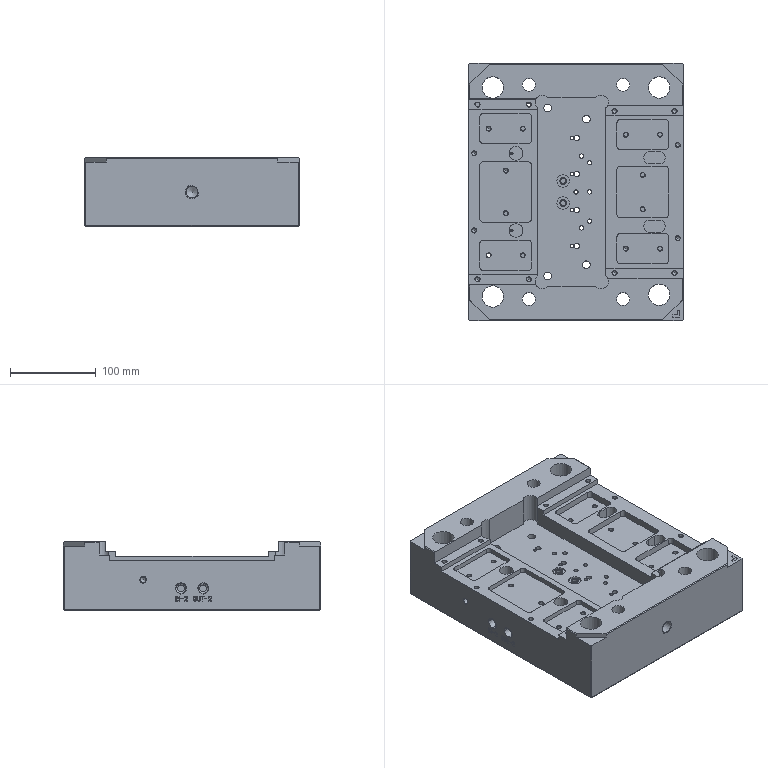NC program | PowerMill | posted with a generic post | part box 250 x 300 x 80 mm
Whole program:
%
O0001
N104 ( POWERMILL CB  : 2026004.0)
N105 ( POST VER      : 2026.0.0.5161)
N106 ( OPTION FILE   : FANUC)
N107 ( OUTPUT WORKPLANE : 1)
N108 (  )
N109 ( TOOL LIST )
N110 (-----------------------------------)
N111 ( NO. | ID    | DIA.| TIP RAD|LENGTH)
N112 (-----------------------------------)
N113 (    1|￠6_1_1| 6.0 |  0.0   |139.96)
N114 (-----------------------------------)
N115 (  )
N116 ( NUMBER OF TOOLPATHS: 1.0 )
N117 ( ESTIMATED PROGRAM DURATION: 0 HOURS 3 MIN 57 SEC)
N118 (  )
N119 G00 G21 G80 G40 G17
N120 G90
N121 G54
N122 G53 Z0.0
N123 (---------------)
N124 ( START TOOLPATH : 04开粗-￠6-钻孔加工 )
N125 (---------------)
N126 ( TOOL NO.    :1 )
N127 ( TOOL TYPE   : DRILL)
N128 ( TOOL ID     : ￠6_1_1)
N129 ( TOOL DIA    : 6.0 LENGTH 139.96)
N130 T1
N131 M6
N132 S700 M03
N133 G00 G90 X63.0 Y-1.0
N134 G43 Z20.0 H1
N135
N136 G05 P10000 R8
N137 Z11.0
N138 G01 Z-2.0 F80.0
N139 G00 Z11.0
N140 Z-1.4
N141 G01 Z-5.0
N142 G00 Z11.0
N143 Z-4.4
N144 G01 Z-8.0
N145 G00 Z11.0
N146 Z-7.4
N147 G01 Z-11.0
N148 G00 Z11.0
N149 Z-10.4
N150 G01 Z-14.0
N151 G00 Z11.0
N152 Z-13.4
N153 G01 Z-17.0
N154 G00 Z11.0
N155 Z-16.4
N156 G01 Z-20.0
N157 G00 Z11.0
N158 Z-19.4
N159 G01 Z-23.0
N160 G00 Z11.0
N161 Z-22.4
N162 G01 Z-26.0
N163 G00 Z11.0
N164 Z-25.4
N165 G01 Z-29.0
N166 G00 Z11.0
N167 Z-28.4
N168 G01 Z-32.0
N169 G00 Z11.0
N170 Z-31.4
N171 G01 Z-35.0
N172 G00 Z11.0
N173 Z-34.4
N174 G01 Z-38.0
N175 G00 Z11.0
N176 Z-37.4
N177 G01 Z-41.0
N178 G00 Z11.0
N179 Z-40.4
N180 G01 Z-44.0
N181 G00 Z11.0
N182 Z-43.4
N183 G01 Z-47.0
N184 G00 Z11.0
N185 Z-46.4
N186 G01 Z-48.7092
N187 G00 Z20.0
N188 X21.0
N189 Z11.0
N190 G01 Z-2.0
N191 G00 Z11.0
N192 Z-1.4
N193 G01 Z-5.0
N194 G00 Z11.0
N195 Z-4.4
N196 G01 Z-8.0
N197 G00 Z11.0
N198 Z-7.4
N199 G01 Z-11.0
N200 G00 Z11.0
N201 Z-10.4
N202 G01 Z-14.0
N203 G00 Z11.0
N204 Z-13.4
N205 G01 Z-17.0
N206 G00 Z11.0
N207 Z-16.4
N208 G01 Z-20.0
N209 G00 Z11.0
N210 Z-19.4
N211 G01 Z-23.0
N212 G00 Z11.0
N213 Z-22.4
N214 G01 Z-26.0
N215 G00 Z11.0
N216 Z-25.4
N217 G01 Z-29.0
N218 G00 Z11.0
N219 Z-28.4
N220 G01 Z-32.0
N221 G00 Z11.0
N222 Z-31.4
N223 G01 Z-35.0
N224 G00 Z11.0
N225 Z-34.4
N226 G01 Z-38.0
N227 G00 Z11.0
N228 Z-37.4
N229 G01 Z-41.0
N230 G00 Z11.0
N231 Z-40.4
N232 G01 Z-44.0
N233 G00 Z11.0
N234 Z-43.4
N235 G01 Z-47.0
N236 G00 Z11.0
N237 Z-46.4
N238 G01 Z-48.7092
N239 G00 Z20.0
N240 X-21.0
N241 Z11.0
N242 G01 Z-2.0
N243 G00 Z11.0
N244 Z-1.4
N245 G01 Z-5.0
N246 G00 Z11.0
N247 Z-4.4
N248 G01 Z-8.0
N249 G00 Z11.0
N250 Z-7.4
N251 G01 Z-11.0
N252 G00 Z11.0
N253 Z-10.4
N254 G01 Z-14.0
N255 G00 Z11.0
N256 Z-13.4
N257 G01 Z-17.0
N258 G00 Z11.0
N259 Z-16.4
N260 G01 Z-20.0
N261 G00 Z11.0
N262 Z-19.4
N263 G01 Z-23.0
N264 G00 Z11.0
N265 Z-22.4
N266 G01 Z-26.0
N267 G00 Z11.0
N268 Z-25.4
N269 G01 Z-29.0
N270 G00 Z11.0
N271 Z-28.4
N272 G01 Z-32.0
N273 G00 Z11.0
N274 Z-31.4
N275 G01 Z-35.0
N276 G00 Z11.0
N277 Z-34.4
N278 G01 Z-38.0
N279 G00 Z11.0
N280 Z-37.4
N281 G01 Z-41.0
N282 G00 Z11.0
N283 Z-40.4
N284 G01 Z-44.0
N285 G00 Z11.0
N286 Z-43.4
N287 G01 Z-47.0
N288 G00 Z11.0
N289 Z-46.4
N290 G01 Z-48.7092
N291 G00 Z20.0
N292 X-63.0
N293 Z11.0
N294 G01 Z-2.0
N295 G00 Z11.0
N296 Z-1.4
N297 G01 Z-5.0
N298 G00 Z11.0
N299 Z-4.4
N300 G01 Z-8.0
N301 G00 Z11.0
N302 Z-7.4
N303 G01 Z-11.0
N304 G00 Z11.0
N305 Z-10.4
N306 G01 Z-14.0
N307 G00 Z11.0
N308 Z-13.4
N309 G01 Z-17.0
N310 G00 Z11.0
N311 Z-16.4
N312 G01 Z-20.0
N313 G00 Z11.0
N314 Z-19.4
N315 G01 Z-23.0
N316 G00 Z11.0
N317 Z-22.4
N318 G01 Z-26.0
N319 G00 Z11.0
N320 Z-25.4
N321 G01 Z-29.0
N322 G00 Z11.0
N323 Z-28.4
N324 G01 Z-32.0
N325 G00 Z11.0
N326 Z-31.4
N327 G01 Z-35.0
N328 G00 Z11.0
N329 Z-34.4
N330 G01 Z-38.0
N331 G00 Z11.0
N332 Z-37.4
N333 G01 Z-41.0
N334 G00 Z11.0
N335 Z-40.4
N336 G01 Z-44.0
N337 G00 Z11.0
N338 Z-43.4
N339 G01 Z-47.0
N340 G00 Z11.0
N341 Z-46.4
N342 G01 Z-48.7092
N343 G00 Z20.0
N344 G05 P0
N345 (---------------)
N346 ( END TOOLPATH : 04开粗-￠6-钻孔加工 )
N347 (---------------)
N348
N349 M05
N350 G53 Z0.0
N351 M30
%